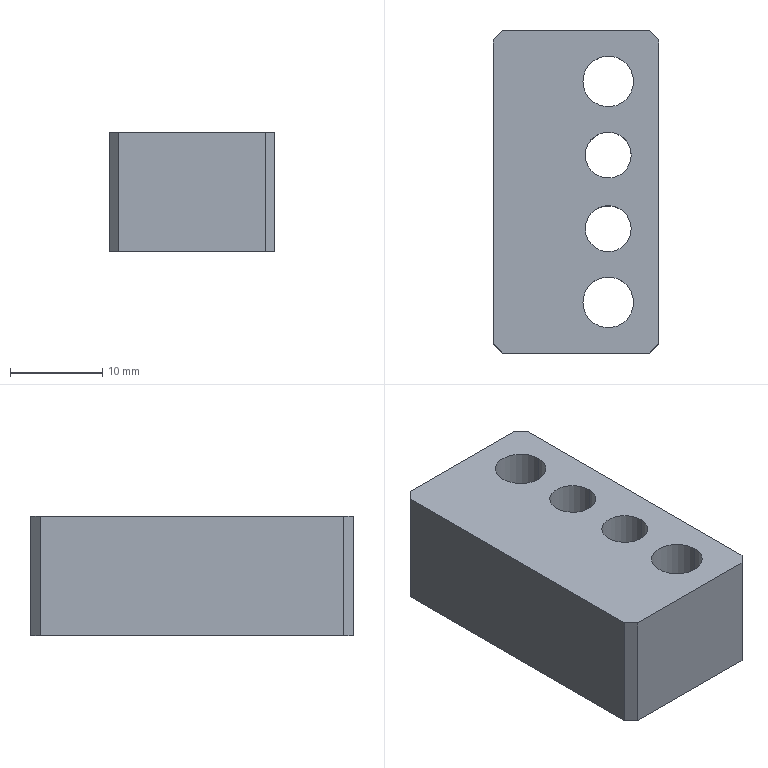Part | STEP file | 11-FG-E01611 | 1 solid | 24 faces | box 18 x 35 x 13 mm | volume 6444 mm3 | cylinder 12 | plane 12 | commonest cylinder face diameters 5 x4 5.5 x4 10 x4
STEP:
#1=CARTESIAN_POINT('',(-8.,21.5,13.));
#2=VERTEX_POINT('',#1);
#3=CARTESIAN_POINT('',(-3.,21.5,13.));
#4=VERTEX_POINT('',#3);
#5=CARTESIAN_POINT('',(-5.5,21.5,13.));
#6=DIRECTION('',(0.,0.,1.));
#7=DIRECTION('',(1.,0.,0.));
#8=AXIS2_PLACEMENT_3D('',#5,#6,#7);
#9=CIRCLE('',#8,2.5);
#10=EDGE_CURVE('',#2,#4,#9,.T.);
#11=ORIENTED_EDGE('',*,*,#10,.T.);
#12=CARTESIAN_POINT('',(-3.,21.5,0.));
#13=VERTEX_POINT('',#12);
#14=CARTESIAN_POINT('',(-3.,21.5,0.));
#15=DIRECTION('',(0.,0.,-1.));
#16=VECTOR('',#15,1000.);
#17=LINE('',#14,#16);
#18=EDGE_CURVE('',#4,#13,#17,.T.);
#19=ORIENTED_EDGE('',*,*,#18,.T.);
#20=CARTESIAN_POINT('',(-8.,21.5,0.));
#21=VERTEX_POINT('',#20);
#22=CARTESIAN_POINT('',(-5.5,21.5,0.));
#23=DIRECTION('',(0.,0.,-1.));
#24=DIRECTION('',(-1.,0.,0.));
#25=AXIS2_PLACEMENT_3D('',#22,#23,#24);
#26=CIRCLE('',#25,2.5);
#27=EDGE_CURVE('',#13,#21,#26,.T.);
#28=ORIENTED_EDGE('',*,*,#27,.T.);
#29=CARTESIAN_POINT('',(-8.,21.5,0.));
#30=DIRECTION('',(0.,0.,-1.));
#31=VECTOR('',#30,1000.);
#32=LINE('',#29,#31);
#33=EDGE_CURVE('',#2,#21,#32,.T.);
#34=ORIENTED_EDGE('',*,*,#33,.F.);
#35=EDGE_LOOP('',(#11,#19,#28,#34));
#36=FACE_OUTER_BOUND('',#35,.T.);
#37=CARTESIAN_POINT('',(-5.5,21.5,0.));
#38=DIRECTION('',(0.,0.,-1.));
#39=DIRECTION('',(-1.,0.,0.));
#40=AXIS2_PLACEMENT_3D('',#37,#38,#39);
#41=CYLINDRICAL_SURFACE('',#40,2.5);
#42=ADVANCED_FACE('',(#36),#41,.F.);
#43=CARTESIAN_POINT('',(-8.,13.5,13.));
#44=VERTEX_POINT('',#43);
#45=CARTESIAN_POINT('',(-3.,13.5,13.));
#46=VERTEX_POINT('',#45);
#47=CARTESIAN_POINT('',(-5.5,13.5,13.));
#48=DIRECTION('',(0.,0.,1.));
#49=DIRECTION('',(1.,0.,0.));
#50=AXIS2_PLACEMENT_3D('',#47,#48,#49);
#51=CIRCLE('',#50,2.5);
#52=EDGE_CURVE('',#44,#46,#51,.T.);
#53=ORIENTED_EDGE('',*,*,#52,.T.);
#54=CARTESIAN_POINT('',(-3.,13.5,0.));
#55=VERTEX_POINT('',#54);
#56=CARTESIAN_POINT('',(-3.,13.5,0.));
#57=DIRECTION('',(0.,0.,-1.));
#58=VECTOR('',#57,1000.);
#59=LINE('',#56,#58);
#60=EDGE_CURVE('',#46,#55,#59,.T.);
#61=ORIENTED_EDGE('',*,*,#60,.T.);
#62=CARTESIAN_POINT('',(-8.,13.5,0.));
#63=VERTEX_POINT('',#62);
#64=CARTESIAN_POINT('',(-5.5,13.5,0.));
#65=DIRECTION('',(0.,0.,-1.));
#66=DIRECTION('',(-1.,0.,0.));
#67=AXIS2_PLACEMENT_3D('',#64,#65,#66);
#68=CIRCLE('',#67,2.5);
#69=EDGE_CURVE('',#55,#63,#68,.T.);
#70=ORIENTED_EDGE('',*,*,#69,.T.);
#71=CARTESIAN_POINT('',(-8.,13.5,0.));
#72=DIRECTION('',(0.,0.,-1.));
#73=VECTOR('',#72,1000.);
#74=LINE('',#71,#73);
#75=EDGE_CURVE('',#44,#63,#74,.T.);
#76=ORIENTED_EDGE('',*,*,#75,.F.);
#77=EDGE_LOOP('',(#53,#61,#70,#76));
#78=FACE_OUTER_BOUND('',#77,.T.);
#79=CARTESIAN_POINT('',(-5.5,13.5,0.));
#80=DIRECTION('',(0.,0.,-1.));
#81=DIRECTION('',(-1.,0.,0.));
#82=AXIS2_PLACEMENT_3D('',#79,#80,#81);
#83=CYLINDRICAL_SURFACE('',#82,2.5);
#84=ADVANCED_FACE('',(#78),#83,.F.);
#85=CARTESIAN_POINT('',(-0.5,29.5,5.4));
#86=VERTEX_POINT('',#85);
#87=CARTESIAN_POINT('',(-10.5,29.5,5.4));
#88=VERTEX_POINT('',#87);
#89=CARTESIAN_POINT('',(-5.5,29.5,5.4));
#90=DIRECTION('',(0.,0.,-1.));
#91=DIRECTION('',(-1.,0.,0.));
#92=AXIS2_PLACEMENT_3D('',#89,#90,#91);
#93=CIRCLE('',#92,5.);
#94=EDGE_CURVE('',#86,#88,#93,.T.);
#95=ORIENTED_EDGE('',*,*,#94,.F.);
#96=CARTESIAN_POINT('',(-0.5,29.5,0.));
#97=VERTEX_POINT('',#96);
#98=CARTESIAN_POINT('',(-0.5,29.5,0.));
#99=DIRECTION('',(0.,0.,-1.));
#100=VECTOR('',#99,1000.);
#101=LINE('',#98,#100);
#102=EDGE_CURVE('',#86,#97,#101,.T.);
#103=ORIENTED_EDGE('',*,*,#102,.T.);
#104=CARTESIAN_POINT('',(-10.5,29.5,0.));
#105=VERTEX_POINT('',#104);
#106=CARTESIAN_POINT('',(-5.5,29.5,0.));
#107=DIRECTION('',(0.,0.,-1.));
#108=DIRECTION('',(-1.,0.,0.));
#109=AXIS2_PLACEMENT_3D('',#106,#107,#108);
#110=CIRCLE('',#109,5.);
#111=EDGE_CURVE('',#97,#105,#110,.T.);
#112=ORIENTED_EDGE('',*,*,#111,.T.);
#113=CARTESIAN_POINT('',(-10.5,29.5,0.));
#114=DIRECTION('',(0.,0.,-1.));
#115=VECTOR('',#114,1000.);
#116=LINE('',#113,#115);
#117=EDGE_CURVE('',#88,#105,#116,.T.);
#118=ORIENTED_EDGE('',*,*,#117,.F.);
#119=EDGE_LOOP('',(#95,#103,#112,#118));
#120=FACE_OUTER_BOUND('',#119,.T.);
#121=CARTESIAN_POINT('',(-5.5,29.5,0.));
#122=DIRECTION('',(0.,0.,-1.));
#123=DIRECTION('',(-1.,0.,0.));
#124=AXIS2_PLACEMENT_3D('',#121,#122,#123);
#125=CYLINDRICAL_SURFACE('',#124,5.);
#126=ADVANCED_FACE('',(#120),#125,.F.);
#127=CARTESIAN_POINT('',(-8.25,29.5,13.));
#128=VERTEX_POINT('',#127);
#129=CARTESIAN_POINT('',(-2.75,29.5,13.));
#130=VERTEX_POINT('',#129);
#131=CARTESIAN_POINT('',(-5.5,29.5,13.));
#132=DIRECTION('',(0.,0.,1.));
#133=DIRECTION('',(1.,0.,0.));
#134=AXIS2_PLACEMENT_3D('',#131,#132,#133);
#135=CIRCLE('',#134,2.75);
#136=EDGE_CURVE('',#128,#130,#135,.T.);
#137=ORIENTED_EDGE('',*,*,#136,.T.);
#138=CARTESIAN_POINT('',(-2.75,29.5,5.4));
#139=VERTEX_POINT('',#138);
#140=CARTESIAN_POINT('',(-2.75,29.5,0.));
#141=DIRECTION('',(0.,0.,-1.));
#142=VECTOR('',#141,1000.);
#143=LINE('',#140,#142);
#144=EDGE_CURVE('',#130,#139,#143,.T.);
#145=ORIENTED_EDGE('',*,*,#144,.T.);
#146=CARTESIAN_POINT('',(-8.25,29.5,5.4));
#147=VERTEX_POINT('',#146);
#148=CARTESIAN_POINT('',(-5.5,29.5,5.4));
#149=DIRECTION('',(0.,0.,-1.));
#150=DIRECTION('',(-1.,0.,0.));
#151=AXIS2_PLACEMENT_3D('',#148,#149,#150);
#152=CIRCLE('',#151,2.75);
#153=EDGE_CURVE('',#139,#147,#152,.T.);
#154=ORIENTED_EDGE('',*,*,#153,.T.);
#155=CARTESIAN_POINT('',(-8.25,29.5,0.));
#156=DIRECTION('',(0.,0.,-1.));
#157=VECTOR('',#156,1000.);
#158=LINE('',#155,#157);
#159=EDGE_CURVE('',#128,#147,#158,.T.);
#160=ORIENTED_EDGE('',*,*,#159,.F.);
#161=EDGE_LOOP('',(#137,#145,#154,#160));
#162=FACE_OUTER_BOUND('',#161,.T.);
#163=CARTESIAN_POINT('',(-5.5,29.5,0.));
#164=DIRECTION('',(0.,0.,-1.));
#165=DIRECTION('',(-1.,0.,0.));
#166=AXIS2_PLACEMENT_3D('',#163,#164,#165);
#167=CYLINDRICAL_SURFACE('',#166,2.75);
#168=ADVANCED_FACE('',(#162),#167,.F.);
#169=CARTESIAN_POINT('',(-0.5,5.5,5.4));
#170=VERTEX_POINT('',#169);
#171=CARTESIAN_POINT('',(-10.5,5.5,5.4));
#172=VERTEX_POINT('',#171);
#173=CARTESIAN_POINT('',(-5.5,5.5,5.4));
#174=DIRECTION('',(0.,0.,-1.));
#175=DIRECTION('',(-1.,0.,0.));
#176=AXIS2_PLACEMENT_3D('',#173,#174,#175);
#177=CIRCLE('',#176,5.);
#178=EDGE_CURVE('',#170,#172,#177,.T.);
#179=ORIENTED_EDGE('',*,*,#178,.F.);
#180=CARTESIAN_POINT('',(-0.5,5.5,0.));
#181=VERTEX_POINT('',#180);
#182=CARTESIAN_POINT('',(-0.5,5.5,0.));
#183=DIRECTION('',(0.,0.,-1.));
#184=VECTOR('',#183,1000.);
#185=LINE('',#182,#184);
#186=EDGE_CURVE('',#170,#181,#185,.T.);
#187=ORIENTED_EDGE('',*,*,#186,.T.);
#188=CARTESIAN_POINT('',(-10.5,5.5,0.));
#189=VERTEX_POINT('',#188);
#190=CARTESIAN_POINT('',(-5.5,5.5,0.));
#191=DIRECTION('',(0.,0.,-1.));
#192=DIRECTION('',(-1.,0.,0.));
#193=AXIS2_PLACEMENT_3D('',#190,#191,#192);
#194=CIRCLE('',#193,5.);
#195=EDGE_CURVE('',#181,#189,#194,.T.);
#196=ORIENTED_EDGE('',*,*,#195,.T.);
#197=CARTESIAN_POINT('',(-10.5,5.5,0.));
#198=DIRECTION('',(0.,0.,-1.));
#199=VECTOR('',#198,1000.);
#200=LINE('',#197,#199);
#201=EDGE_CURVE('',#172,#189,#200,.T.);
#202=ORIENTED_EDGE('',*,*,#201,.F.);
#203=EDGE_LOOP('',(#179,#187,#196,#202));
#204=FACE_OUTER_BOUND('',#203,.T.);
#205=CARTESIAN_POINT('',(-5.5,5.5,0.));
#206=DIRECTION('',(0.,0.,-1.));
#207=DIRECTION('',(-1.,0.,0.));
#208=AXIS2_PLACEMENT_3D('',#205,#206,#207);
#209=CYLINDRICAL_SURFACE('',#208,5.);
#210=ADVANCED_FACE('',(#204),#209,.F.);
#211=CARTESIAN_POINT('',(-8.25,5.5,13.));
#212=VERTEX_POINT('',#211);
#213=CARTESIAN_POINT('',(-2.75,5.5,13.));
#214=VERTEX_POINT('',#213);
#215=CARTESIAN_POINT('',(-5.5,5.5,13.));
#216=DIRECTION('',(0.,0.,1.));
#217=DIRECTION('',(1.,0.,0.));
#218=AXIS2_PLACEMENT_3D('',#215,#216,#217);
#219=CIRCLE('',#218,2.75);
#220=EDGE_CURVE('',#212,#214,#219,.T.);
#221=ORIENTED_EDGE('',*,*,#220,.T.);
#222=CARTESIAN_POINT('',(-2.75,5.5,5.4));
#223=VERTEX_POINT('',#222);
#224=CARTESIAN_POINT('',(-2.75,5.5,0.));
#225=DIRECTION('',(0.,0.,-1.));
#226=VECTOR('',#225,1000.);
#227=LINE('',#224,#226);
#228=EDGE_CURVE('',#214,#223,#227,.T.);
#229=ORIENTED_EDGE('',*,*,#228,.T.);
#230=CARTESIAN_POINT('',(-8.25,5.5,5.4));
#231=VERTEX_POINT('',#230);
#232=CARTESIAN_POINT('',(-5.5,5.5,5.4));
#233=DIRECTION('',(0.,0.,-1.));
#234=DIRECTION('',(-1.,0.,0.));
#235=AXIS2_PLACEMENT_3D('',#232,#233,#234);
#236=CIRCLE('',#235,2.75);
#237=EDGE_CURVE('',#223,#231,#236,.T.);
#238=ORIENTED_EDGE('',*,*,#237,.T.);
#239=CARTESIAN_POINT('',(-8.25,5.5,0.));
#240=DIRECTION('',(0.,0.,-1.));
#241=VECTOR('',#240,1000.);
#242=LINE('',#239,#241);
#243=EDGE_CURVE('',#212,#231,#242,.T.);
#244=ORIENTED_EDGE('',*,*,#243,.F.);
#245=EDGE_LOOP('',(#221,#229,#238,#244));
#246=FACE_OUTER_BOUND('',#245,.T.);
#247=CARTESIAN_POINT('',(-5.5,5.5,0.));
#248=DIRECTION('',(0.,0.,-1.));
#249=DIRECTION('',(-1.,0.,0.));
#250=AXIS2_PLACEMENT_3D('',#247,#248,#249);
#251=CYLINDRICAL_SURFACE('',#250,2.75);
#252=ADVANCED_FACE('',(#246),#251,.F.);
#253=CARTESIAN_POINT('',(0.,1.,13.));
#254=VERTEX_POINT('',#253);
#255=CARTESIAN_POINT('',(0.,34.,13.));
#256=VERTEX_POINT('',#255);
#257=CARTESIAN_POINT('',(0.,0.,13.));
#258=DIRECTION('',(0.,1.,0.));
#259=VECTOR('',#258,1000.);
#260=LINE('',#257,#259);
#261=EDGE_CURVE('',#254,#256,#260,.T.);
#262=ORIENTED_EDGE('',*,*,#261,.F.);
#263=CARTESIAN_POINT('',(0.,1.,0.));
#264=VERTEX_POINT('',#263);
#265=CARTESIAN_POINT('',(0.,1.,13.));
#266=DIRECTION('',(0.,0.,-1.));
#267=VECTOR('',#266,1000.);
#268=LINE('',#265,#267);
#269=EDGE_CURVE('',#254,#264,#268,.T.);
#270=ORIENTED_EDGE('',*,*,#269,.T.);
#271=CARTESIAN_POINT('',(0.,34.,0.));
#272=VERTEX_POINT('',#271);
#273=CARTESIAN_POINT('',(0.,0.,0.));
#274=DIRECTION('',(0.,1.,0.));
#275=VECTOR('',#274,1000.);
#276=LINE('',#273,#275);
#277=EDGE_CURVE('',#264,#272,#276,.T.);
#278=ORIENTED_EDGE('',*,*,#277,.T.);
#279=CARTESIAN_POINT('',(0.,34.,13.));
#280=DIRECTION('',(0.,0.,1.));
#281=VECTOR('',#280,1000.);
#282=LINE('',#279,#281);
#283=EDGE_CURVE('',#272,#256,#282,.T.);
#284=ORIENTED_EDGE('',*,*,#283,.T.);
#285=EDGE_LOOP('',(#262,#270,#278,#284));
#286=FACE_OUTER_BOUND('',#285,.T.);
#287=CARTESIAN_POINT('',(0.,0.,13.));
#288=DIRECTION('',(-1.,0.,0.));
#289=DIRECTION('',(0.,0.,1.));
#290=AXIS2_PLACEMENT_3D('',#287,#288,#289);
#291=PLANE('',#290);
#292=ADVANCED_FACE('',(#286),#291,.F.);
#293=CARTESIAN_POINT('',(-1.,35.,13.));
#294=VERTEX_POINT('',#293);
#295=CARTESIAN_POINT('',(-17.,35.,13.));
#296=VERTEX_POINT('',#295);
#297=CARTESIAN_POINT('',(0.,35.,13.));
#298=DIRECTION('',(-1.,0.,0.));
#299=VECTOR('',#298,1000.);
#300=LINE('',#297,#299);
#301=EDGE_CURVE('',#294,#296,#300,.T.);
#302=ORIENTED_EDGE('',*,*,#301,.F.);
#303=CARTESIAN_POINT('',(-1.,35.,0.));
#304=VERTEX_POINT('',#303);
#305=CARTESIAN_POINT('',(-1.,35.,13.));
#306=DIRECTION('',(0.,0.,-1.));
#307=VECTOR('',#306,1000.);
#308=LINE('',#305,#307);
#309=EDGE_CURVE('',#294,#304,#308,.T.);
#310=ORIENTED_EDGE('',*,*,#309,.T.);
#311=CARTESIAN_POINT('',(-17.,35.,0.));
#312=VERTEX_POINT('',#311);
#313=CARTESIAN_POINT('',(0.,35.,0.));
#314=DIRECTION('',(-1.,0.,0.));
#315=VECTOR('',#314,1000.);
#316=LINE('',#313,#315);
#317=EDGE_CURVE('',#304,#312,#316,.T.);
#318=ORIENTED_EDGE('',*,*,#317,.T.);
#319=CARTESIAN_POINT('',(-17.,35.,13.));
#320=DIRECTION('',(0.,0.,1.));
#321=VECTOR('',#320,1000.);
#322=LINE('',#319,#321);
#323=EDGE_CURVE('',#312,#296,#322,.T.);
#324=ORIENTED_EDGE('',*,*,#323,.T.);
#325=EDGE_LOOP('',(#302,#310,#318,#324));
#326=FACE_OUTER_BOUND('',#325,.T.);
#327=CARTESIAN_POINT('',(0.,35.,13.));
#328=DIRECTION('',(0.,-1.,0.));
#329=DIRECTION('',(1.,0.,0.));
#330=AXIS2_PLACEMENT_3D('',#327,#328,#329);
#331=PLANE('',#330);
#332=ADVANCED_FACE('',(#326),#331,.F.);
#333=CARTESIAN_POINT('',(-18.,34.,0.));
#334=VERTEX_POINT('',#333);
#335=CARTESIAN_POINT('',(-18.,1.,0.));
#336=VERTEX_POINT('',#335);
#337=CARTESIAN_POINT('',(-18.,0.,0.));
#338=DIRECTION('',(0.,-1.,0.));
#339=VECTOR('',#338,1000.);
#340=LINE('',#337,#339);
#341=EDGE_CURVE('',#334,#336,#340,.T.);
#342=ORIENTED_EDGE('',*,*,#341,.T.);
#343=CARTESIAN_POINT('',(-18.,1.,13.));
#344=VERTEX_POINT('',#343);
#345=CARTESIAN_POINT('',(-18.,1.,13.));
#346=DIRECTION('',(0.,0.,1.));
#347=VECTOR('',#346,1000.);
#348=LINE('',#345,#347);
#349=EDGE_CURVE('',#336,#344,#348,.T.);
#350=ORIENTED_EDGE('',*,*,#349,.T.);
#351=CARTESIAN_POINT('',(-18.,34.,13.));
#352=VERTEX_POINT('',#351);
#353=CARTESIAN_POINT('',(-18.,0.,13.));
#354=DIRECTION('',(0.,-1.,0.));
#355=VECTOR('',#354,1000.);
#356=LINE('',#353,#355);
#357=EDGE_CURVE('',#352,#344,#356,.T.);
#358=ORIENTED_EDGE('',*,*,#357,.F.);
#359=CARTESIAN_POINT('',(-18.,34.,13.));
#360=DIRECTION('',(0.,0.,-1.));
#361=VECTOR('',#360,1000.);
#362=LINE('',#359,#361);
#363=EDGE_CURVE('',#352,#334,#362,.T.);
#364=ORIENTED_EDGE('',*,*,#363,.T.);
#365=EDGE_LOOP('',(#342,#350,#358,#364));
#366=FACE_OUTER_BOUND('',#365,.T.);
#367=CARTESIAN_POINT('',(-18.,0.,13.));
#368=DIRECTION('',(1.,0.,0.));
#369=DIRECTION('',(0.,0.,-1.));
#370=AXIS2_PLACEMENT_3D('',#367,#368,#369);
#371=PLANE('',#370);
#372=ADVANCED_FACE('',(#366),#371,.F.);
#373=CARTESIAN_POINT('',(-17.,0.,0.));
#374=VERTEX_POINT('',#373);
#375=CARTESIAN_POINT('',(-1.,0.,0.));
#376=VERTEX_POINT('',#375);
#377=CARTESIAN_POINT('',(0.,0.,0.));
#378=DIRECTION('',(1.,0.,0.));
#379=VECTOR('',#378,1000.);
#380=LINE('',#377,#379);
#381=EDGE_CURVE('',#374,#376,#380,.T.);
#382=ORIENTED_EDGE('',*,*,#381,.T.);
#383=CARTESIAN_POINT('',(-1.,0.,13.));
#384=VERTEX_POINT('',#383);
#385=CARTESIAN_POINT('',(-1.,0.,13.));
#386=DIRECTION('',(0.,0.,1.));
#387=VECTOR('',#386,1000.);
#388=LINE('',#385,#387);
#389=EDGE_CURVE('',#376,#384,#388,.T.);
#390=ORIENTED_EDGE('',*,*,#389,.T.);
#391=CARTESIAN_POINT('',(-17.,0.,13.));
#392=VERTEX_POINT('',#391);
#393=CARTESIAN_POINT('',(0.,0.,13.));
#394=DIRECTION('',(1.,0.,0.));
#395=VECTOR('',#394,1000.);
#396=LINE('',#393,#395);
#397=EDGE_CURVE('',#392,#384,#396,.T.);
#398=ORIENTED_EDGE('',*,*,#397,.F.);
#399=CARTESIAN_POINT('',(-17.,0.,13.));
#400=DIRECTION('',(0.,0.,-1.));
#401=VECTOR('',#400,1000.);
#402=LINE('',#399,#401);
#403=EDGE_CURVE('',#392,#374,#402,.T.);
#404=ORIENTED_EDGE('',*,*,#403,.T.);
#405=EDGE_LOOP('',(#382,#390,#398,#404));
#406=FACE_OUTER_BOUND('',#405,.T.);
#407=CARTESIAN_POINT('',(0.,0.,13.));
#408=DIRECTION('',(0.,1.,0.));
#409=DIRECTION('',(-1.,0.,0.));
#410=AXIS2_PLACEMENT_3D('',#407,#408,#409);
#411=PLANE('',#410);
#412=ADVANCED_FACE('',(#406),#411,.F.);
#413=ORIENTED_EDGE('',*,*,#10,.F.);
#414=CARTESIAN_POINT('',(-5.5,21.5,13.));
#415=DIRECTION('',(0.,0.,1.));
#416=DIRECTION('',(1.,0.,0.));
#417=AXIS2_PLACEMENT_3D('',#414,#415,#416);
#418=CIRCLE('',#417,2.5);
#419=EDGE_CURVE('',#4,#2,#418,.T.);
#420=ORIENTED_EDGE('',*,*,#419,.F.);
#421=EDGE_LOOP('',(#413,#420));
#422=FACE_BOUND('',#421,.T.);
#423=ORIENTED_EDGE('',*,*,#52,.F.);
#424=CARTESIAN_POINT('',(-5.5,13.5,13.));
#425=DIRECTION('',(0.,0.,1.));
#426=DIRECTION('',(1.,0.,0.));
#427=AXIS2_PLACEMENT_3D('',#424,#425,#426);
#428=CIRCLE('',#427,2.5);
#429=EDGE_CURVE('',#46,#44,#428,.T.);
#430=ORIENTED_EDGE('',*,*,#429,.F.);
#431=EDGE_LOOP('',(#423,#430));
#432=FACE_BOUND('',#431,.T.);
#433=ORIENTED_EDGE('',*,*,#136,.F.);
#434=CARTESIAN_POINT('',(-5.5,29.5,13.));
#435=DIRECTION('',(0.,0.,1.));
#436=DIRECTION('',(1.,0.,0.));
#437=AXIS2_PLACEMENT_3D('',#434,#435,#436);
#438=CIRCLE('',#437,2.75);
#439=EDGE_CURVE('',#130,#128,#438,.T.);
#440=ORIENTED_EDGE('',*,*,#439,.F.);
#441=EDGE_LOOP('',(#433,#440));
#442=FACE_BOUND('',#441,.T.);
#443=ORIENTED_EDGE('',*,*,#220,.F.);
#444=CARTESIAN_POINT('',(-5.5,5.5,13.));
#445=DIRECTION('',(0.,0.,1.));
#446=DIRECTION('',(1.,0.,0.));
#447=AXIS2_PLACEMENT_3D('',#444,#445,#446);
#448=CIRCLE('',#447,2.75);
#449=EDGE_CURVE('',#214,#212,#448,.T.);
#450=ORIENTED_EDGE('',*,*,#449,.F.);
#451=EDGE_LOOP('',(#443,#450));
#452=FACE_BOUND('',#451,.T.);
#453=ORIENTED_EDGE('',*,*,#397,.T.);
#454=CARTESIAN_POINT('',(17.,18.,13.));
#455=DIRECTION('',(0.7071,0.7071,0.));
#456=VECTOR('',#455,1000.);
#457=LINE('',#454,#456);
#458=EDGE_CURVE('',#384,#254,#457,.T.);
#459=ORIENTED_EDGE('',*,*,#458,.T.);
#460=ORIENTED_EDGE('',*,*,#261,.T.);
#461=CARTESIAN_POINT('',(-0.5,34.5,13.));
#462=DIRECTION('',(-0.7071,0.7071,0.));
#463=VECTOR('',#462,1000.);
#464=LINE('',#461,#463);
#465=EDGE_CURVE('',#256,#294,#464,.T.);
#466=ORIENTED_EDGE('',*,*,#465,.T.);
#467=ORIENTED_EDGE('',*,*,#301,.T.);
#468=CARTESIAN_POINT('',(-8.5,43.5,13.));
#469=DIRECTION('',(-0.7071,-0.7071,0.));
#470=VECTOR('',#469,1000.);
#471=LINE('',#468,#470);
#472=EDGE_CURVE('',#296,#352,#471,.T.);
#473=ORIENTED_EDGE('',*,*,#472,.T.);
#474=ORIENTED_EDGE('',*,*,#357,.T.);
#475=CARTESIAN_POINT('',(-26.,9.,13.));
#476=DIRECTION('',(0.7071,-0.7071,0.));
#477=VECTOR('',#476,1000.);
#478=LINE('',#475,#477);
#479=EDGE_CURVE('',#344,#392,#478,.T.);
#480=ORIENTED_EDGE('',*,*,#479,.T.);
#481=EDGE_LOOP('',(#453,#459,#460,#466,#467,#473,#474,#480));
#482=FACE_OUTER_BOUND('',#481,.T.);
#483=CARTESIAN_POINT('',(0.,35.,13.));
#484=DIRECTION('',(0.,0.,1.));
#485=DIRECTION('',(1.,0.,0.));
#486=AXIS2_PLACEMENT_3D('',#483,#484,#485);
#487=PLANE('',#486);
#488=ADVANCED_FACE('',(#422,#432,#442,#452,#482),#487,.T.);
#489=CARTESIAN_POINT('',(-5.5,21.5,0.));
#490=DIRECTION('',(0.,0.,-1.));
#491=DIRECTION('',(-1.,0.,0.));
#492=AXIS2_PLACEMENT_3D('',#489,#490,#491);
#493=CIRCLE('',#492,2.5);
#494=EDGE_CURVE('',#21,#13,#493,.T.);
#495=ORIENTED_EDGE('',*,*,#494,.F.);
#496=ORIENTED_EDGE('',*,*,#27,.F.);
#497=EDGE_LOOP('',(#495,#496));
#498=FACE_BOUND('',#497,.T.);
#499=CARTESIAN_POINT('',(-5.5,13.5,0.));
#500=DIRECTION('',(0.,0.,-1.));
#501=DIRECTION('',(-1.,0.,0.));
#502=AXIS2_PLACEMENT_3D('',#499,#500,#501);
#503=CIRCLE('',#502,2.5);
#504=EDGE_CURVE('',#63,#55,#503,.T.);
#505=ORIENTED_EDGE('',*,*,#504,.F.);
#506=ORIENTED_EDGE('',*,*,#69,.F.);
#507=EDGE_LOOP('',(#505,#506));
#508=FACE_BOUND('',#507,.T.);
#509=CARTESIAN_POINT('',(-5.5,29.5,0.));
#510=DIRECTION('',(0.,0.,-1.));
#511=DIRECTION('',(-1.,0.,0.));
#512=AXIS2_PLACEMENT_3D('',#509,#510,#511);
#513=CIRCLE('',#512,5.);
#514=EDGE_CURVE('',#105,#97,#513,.T.);
#515=ORIENTED_EDGE('',*,*,#514,.F.);
#516=ORIENTED_EDGE('',*,*,#111,.F.);
#517=EDGE_LOOP('',(#515,#516));
#518=FACE_BOUND('',#517,.T.);
#519=CARTESIAN_POINT('',(-5.5,5.5,0.));
#520=DIRECTION('',(0.,0.,-1.));
#521=DIRECTION('',(-1.,0.,0.));
#522=AXIS2_PLACEMENT_3D('',#519,#520,#521);
#523=CIRCLE('',#522,5.);
#524=EDGE_CURVE('',#189,#181,#523,.T.);
#525=ORIENTED_EDGE('',*,*,#524,.F.);
#526=ORIENTED_EDGE('',*,*,#195,.F.);
#527=EDGE_LOOP('',(#525,#526));
#528=FACE_BOUND('',#527,.T.);
#529=ORIENTED_EDGE('',*,*,#277,.F.);
#530=CARTESIAN_POINT('',(0.,1.,0.));
#531=DIRECTION('',(-0.7071,-0.7071,0.));
#532=VECTOR('',#531,1000.);
#533=LINE('',#530,#532);
#534=EDGE_CURVE('',#264,#376,#533,.T.);
#535=ORIENTED_EDGE('',*,*,#534,.T.);
#536=ORIENTED_EDGE('',*,*,#381,.F.);
#537=CARTESIAN_POINT('',(-17.,0.,0.));
#538=DIRECTION('',(-0.7071,0.7071,0.));
#539=VECTOR('',#538,1000.);
#540=LINE('',#537,#539);
#541=EDGE_CURVE('',#374,#336,#540,.T.);
#542=ORIENTED_EDGE('',*,*,#541,.T.);
#543=ORIENTED_EDGE('',*,*,#341,.F.);
#544=CARTESIAN_POINT('',(-18.,34.,0.));
#545=DIRECTION('',(0.7071,0.7071,0.));
#546=VECTOR('',#545,1000.);
#547=LINE('',#544,#546);
#548=EDGE_CURVE('',#334,#312,#547,.T.);
#549=ORIENTED_EDGE('',*,*,#548,.T.);
#550=ORIENTED_EDGE('',*,*,#317,.F.);
#551=CARTESIAN_POINT('',(-1.,35.,0.));
#552=DIRECTION('',(0.7071,-0.7071,0.));
#553=VECTOR('',#552,1000.);
#554=LINE('',#551,#553);
#555=EDGE_CURVE('',#304,#272,#554,.T.);
#556=ORIENTED_EDGE('',*,*,#555,.T.);
#557=EDGE_LOOP('',(#529,#535,#536,#542,#543,#549,#550,#556));
#558=FACE_OUTER_BOUND('',#557,.T.);
#559=CARTESIAN_POINT('',(0.,35.,0.));
#560=DIRECTION('',(0.,0.,1.));
#561=DIRECTION('',(1.,0.,0.));
#562=AXIS2_PLACEMENT_3D('',#559,#560,#561);
#563=PLANE('',#562);
#564=ADVANCED_FACE('',(#498,#508,#518,#528,#558),#563,.F.);
#565=ORIENTED_EDGE('',*,*,#228,.F.);
#566=ORIENTED_EDGE('',*,*,#449,.T.);
#567=ORIENTED_EDGE('',*,*,#243,.T.);
#568=CARTESIAN_POINT('',(-5.5,5.5,5.4));
#569=DIRECTION('',(0.,0.,-1.));
#570=DIRECTION('',(-1.,0.,0.));
#571=AXIS2_PLACEMENT_3D('',#568,#569,#570);
#572=CIRCLE('',#571,2.75);
#573=EDGE_CURVE('',#231,#223,#572,.T.);
#574=ORIENTED_EDGE('',*,*,#573,.T.);
#575=EDGE_LOOP('',(#565,#566,#567,#574));
#576=FACE_OUTER_BOUND('',#575,.T.);
#577=CARTESIAN_POINT('',(-5.5,5.5,0.));
#578=DIRECTION('',(0.,0.,-1.));
#579=DIRECTION('',(-1.,0.,0.));
#580=AXIS2_PLACEMENT_3D('',#577,#578,#579);
#581=CYLINDRICAL_SURFACE('',#580,2.75);
#582=ADVANCED_FACE('',(#576),#581,.F.);
#583=ORIENTED_EDGE('',*,*,#573,.F.);
#584=ORIENTED_EDGE('',*,*,#237,.F.);
#585=EDGE_LOOP('',(#583,#584));
#586=FACE_BOUND('',#585,.T.);
#587=CARTESIAN_POINT('',(-5.5,5.5,5.4));
#588=DIRECTION('',(0.,0.,-1.));
#589=DIRECTION('',(-1.,0.,0.));
#590=AXIS2_PLACEMENT_3D('',#587,#588,#589);
#591=CIRCLE('',#590,5.);
#592=EDGE_CURVE('',#172,#170,#591,.T.);
#593=ORIENTED_EDGE('',*,*,#592,.T.);
#594=ORIENTED_EDGE('',*,*,#178,.T.);
#595=EDGE_LOOP('',(#593,#594));
#596=FACE_OUTER_BOUND('',#595,.T.);
#597=CARTESIAN_POINT('',(-2.75,5.5,5.4));
#598=DIRECTION('',(0.,0.,1.));
#599=DIRECTION('',(1.,0.,0.));
#600=AXIS2_PLACEMENT_3D('',#597,#598,#599);
#601=PLANE('',#600);
#602=ADVANCED_FACE('',(#586,#596),#601,.F.);
#603=ORIENTED_EDGE('',*,*,#186,.F.);
#604=ORIENTED_EDGE('',*,*,#592,.F.);
#605=ORIENTED_EDGE('',*,*,#201,.T.);
#606=ORIENTED_EDGE('',*,*,#524,.T.);
#607=EDGE_LOOP('',(#603,#604,#605,#606));
#608=FACE_OUTER_BOUND('',#607,.T.);
#609=CARTESIAN_POINT('',(-5.5,5.5,0.));
#610=DIRECTION('',(0.,0.,-1.));
#611=DIRECTION('',(-1.,0.,0.));
#612=AXIS2_PLACEMENT_3D('',#609,#610,#611);
#613=CYLINDRICAL_SURFACE('',#612,5.);
#614=ADVANCED_FACE('',(#608),#613,.F.);
#615=ORIENTED_EDGE('',*,*,#144,.F.);
#616=ORIENTED_EDGE('',*,*,#439,.T.);
#617=ORIENTED_EDGE('',*,*,#159,.T.);
#618=CARTESIAN_POINT('',(-5.5,29.5,5.4));
#619=DIRECTION('',(0.,0.,-1.));
#620=DIRECTION('',(-1.,0.,0.));
#621=AXIS2_PLACEMENT_3D('',#618,#619,#620);
#622=CIRCLE('',#621,2.75);
#623=EDGE_CURVE('',#147,#139,#622,.T.);
#624=ORIENTED_EDGE('',*,*,#623,.T.);
#625=EDGE_LOOP('',(#615,#616,#617,#624));
#626=FACE_OUTER_BOUND('',#625,.T.);
#627=CARTESIAN_POINT('',(-5.5,29.5,0.));
#628=DIRECTION('',(0.,0.,-1.));
#629=DIRECTION('',(-1.,0.,0.));
#630=AXIS2_PLACEMENT_3D('',#627,#628,#629);
#631=CYLINDRICAL_SURFACE('',#630,2.75);
#632=ADVANCED_FACE('',(#626),#631,.F.);
#633=ORIENTED_EDGE('',*,*,#623,.F.);
#634=ORIENTED_EDGE('',*,*,#153,.F.);
#635=EDGE_LOOP('',(#633,#634));
#636=FACE_BOUND('',#635,.T.);
#637=CARTESIAN_POINT('',(-5.5,29.5,5.4));
#638=DIRECTION('',(0.,0.,-1.));
#639=DIRECTION('',(-1.,0.,0.));
#640=AXIS2_PLACEMENT_3D('',#637,#638,#639);
#641=CIRCLE('',#640,5.);
#642=EDGE_CURVE('',#88,#86,#641,.T.);
#643=ORIENTED_EDGE('',*,*,#642,.T.);
#644=ORIENTED_EDGE('',*,*,#94,.T.);
#645=EDGE_LOOP('',(#643,#644));
#646=FACE_OUTER_BOUND('',#645,.T.);
#647=CARTESIAN_POINT('',(-2.75,29.5,5.4));
#648=DIRECTION('',(0.,0.,1.));
#649=DIRECTION('',(1.,0.,0.));
#650=AXIS2_PLACEMENT_3D('',#647,#648,#649);
#651=PLANE('',#650);
#652=ADVANCED_FACE('',(#636,#646),#651,.F.);
#653=ORIENTED_EDGE('',*,*,#102,.F.);
#654=ORIENTED_EDGE('',*,*,#642,.F.);
#655=ORIENTED_EDGE('',*,*,#117,.T.);
#656=ORIENTED_EDGE('',*,*,#514,.T.);
#657=EDGE_LOOP('',(#653,#654,#655,#656));
#658=FACE_OUTER_BOUND('',#657,.T.);
#659=CARTESIAN_POINT('',(-5.5,29.5,0.));
#660=DIRECTION('',(0.,0.,-1.));
#661=DIRECTION('',(-1.,0.,0.));
#662=AXIS2_PLACEMENT_3D('',#659,#660,#661);
#663=CYLINDRICAL_SURFACE('',#662,5.);
#664=ADVANCED_FACE('',(#658),#663,.F.);
#665=ORIENTED_EDGE('',*,*,#458,.F.);
#666=ORIENTED_EDGE('',*,*,#389,.F.);
#667=ORIENTED_EDGE('',*,*,#534,.F.);
#668=ORIENTED_EDGE('',*,*,#269,.F.);
#669=EDGE_LOOP('',(#665,#666,#667,#668));
#670=FACE_OUTER_BOUND('',#669,.T.);
#671=CARTESIAN_POINT('',(0.,1.,13.));
#672=DIRECTION('',(-0.7071,0.7071,0.));
#673=DIRECTION('',(0.,0.,-1.));
#674=AXIS2_PLACEMENT_3D('',#671,#672,#673);
#675=PLANE('',#674);
#676=ADVANCED_FACE('',(#670),#675,.F.);
#677=ORIENTED_EDGE('',*,*,#479,.F.);
#678=ORIENTED_EDGE('',*,*,#349,.F.);
#679=ORIENTED_EDGE('',*,*,#541,.F.);
#680=ORIENTED_EDGE('',*,*,#403,.F.);
#681=EDGE_LOOP('',(#677,#678,#679,#680));
#682=FACE_OUTER_BOUND('',#681,.T.);
#683=CARTESIAN_POINT('',(-17.,0.,13.));
#684=DIRECTION('',(0.7071,0.7071,0.));
#685=DIRECTION('',(0.,0.,-1.));
#686=AXIS2_PLACEMENT_3D('',#683,#684,#685);
#687=PLANE('',#686);
#688=ADVANCED_FACE('',(#682),#687,.F.);
#689=ORIENTED_EDGE('',*,*,#465,.F.);
#690=ORIENTED_EDGE('',*,*,#283,.F.);
#691=ORIENTED_EDGE('',*,*,#555,.F.);
#692=ORIENTED_EDGE('',*,*,#309,.F.);
#693=EDGE_LOOP('',(#689,#690,#691,#692));
#694=FACE_OUTER_BOUND('',#693,.T.);
#695=CARTESIAN_POINT('',(-1.,35.,13.));
#696=DIRECTION('',(-0.7071,-0.7071,0.));
#697=DIRECTION('',(0.,0.,-1.));
#698=AXIS2_PLACEMENT_3D('',#695,#696,#697);
#699=PLANE('',#698);
#700=ADVANCED_FACE('',(#694),#699,.F.);
#701=ORIENTED_EDGE('',*,*,#472,.F.);
#702=ORIENTED_EDGE('',*,*,#323,.F.);
#703=ORIENTED_EDGE('',*,*,#548,.F.);
#704=ORIENTED_EDGE('',*,*,#363,.F.);
#705=EDGE_LOOP('',(#701,#702,#703,#704));
#706=FACE_OUTER_BOUND('',#705,.T.);
#707=CARTESIAN_POINT('',(-18.,34.,13.));
#708=DIRECTION('',(0.7071,-0.7071,0.));
#709=DIRECTION('',(0.,0.,-1.));
#710=AXIS2_PLACEMENT_3D('',#707,#708,#709);
#711=PLANE('',#710);
#712=ADVANCED_FACE('',(#706),#711,.F.);
#713=ORIENTED_EDGE('',*,*,#60,.F.);
#714=ORIENTED_EDGE('',*,*,#429,.T.);
#715=ORIENTED_EDGE('',*,*,#75,.T.);
#716=ORIENTED_EDGE('',*,*,#504,.T.);
#717=EDGE_LOOP('',(#713,#714,#715,#716));
#718=FACE_OUTER_BOUND('',#717,.T.);
#719=CARTESIAN_POINT('',(-5.5,13.5,0.));
#720=DIRECTION('',(0.,0.,-1.));
#721=DIRECTION('',(-1.,0.,0.));
#722=AXIS2_PLACEMENT_3D('',#719,#720,#721);
#723=CYLINDRICAL_SURFACE('',#722,2.5);
#724=ADVANCED_FACE('',(#718),#723,.F.);
#725=ORIENTED_EDGE('',*,*,#18,.F.);
#726=ORIENTED_EDGE('',*,*,#419,.T.);
#727=ORIENTED_EDGE('',*,*,#33,.T.);
#728=ORIENTED_EDGE('',*,*,#494,.T.);
#729=EDGE_LOOP('',(#725,#726,#727,#728));
#730=FACE_OUTER_BOUND('',#729,.T.);
#731=CARTESIAN_POINT('',(-5.5,21.5,0.));
#732=DIRECTION('',(0.,0.,-1.));
#733=DIRECTION('',(-1.,0.,0.));
#734=AXIS2_PLACEMENT_3D('',#731,#732,#733);
#735=CYLINDRICAL_SURFACE('',#734,2.5);
#736=ADVANCED_FACE('',(#730),#735,.F.);
#737=CLOSED_SHELL('',(#42,#84,#126,#168,#210,#252,#292,#332,#372,#412,#488,#564,#582,#602,#614,#632,#652,#664,#676,#688,#700,#712,#724,#736));
#738=MANIFOLD_SOLID_BREP('',#737);
#739=CARTESIAN_POINT('',(0.,0.,0.));
#740=DIRECTION('',(0.,0.,1.));
#741=DIRECTION('',(1.,0.,0.));
#742=AXIS2_PLACEMENT_3D('',#739,#740,#741);
#743=(LENGTH_UNIT()NAMED_UNIT(*)SI_UNIT(.MILLI.,.METRE.));
#744=UNCERTAINTY_MEASURE_WITH_UNIT(LENGTH_MEASURE(0.00001),#743,'','');
#745=(NAMED_UNIT(*)PLANE_ANGLE_UNIT()SI_UNIT($,.RADIAN.));
#746=(NAMED_UNIT(*)SI_UNIT($,.STERADIAN.)SOLID_ANGLE_UNIT());
#747=(GEOMETRIC_REPRESENTATION_CONTEXT(3)GLOBAL_UNCERTAINTY_ASSIGNED_CONTEXT((#744))GLOBAL_UNIT_ASSIGNED_CONTEXT((#743,#745,#746))REPRESENTATION_CONTEXT('',''));
#748=ADVANCED_BREP_SHAPE_REPRESENTATION('',(#738,#742),#747);